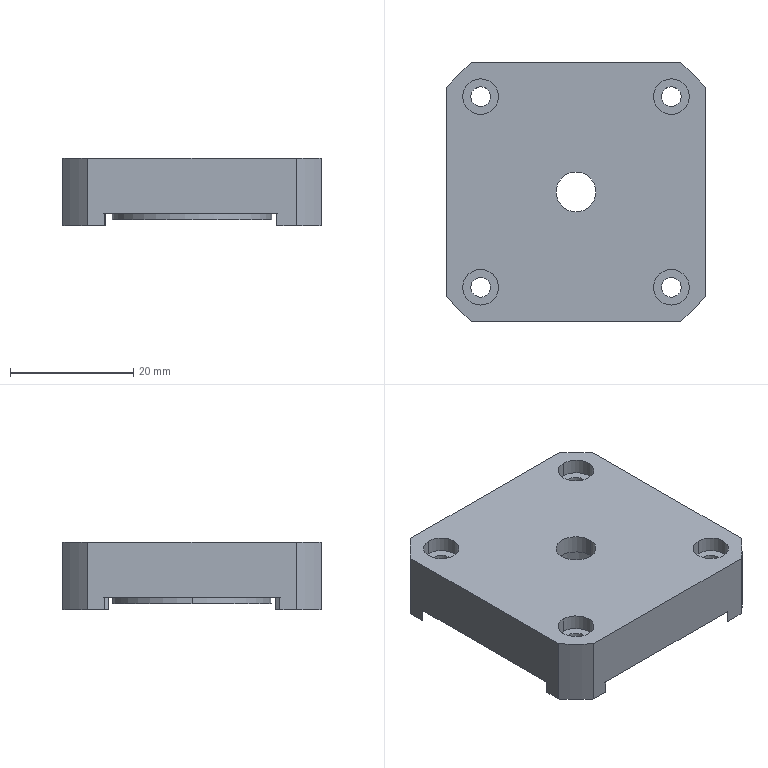Part | SolidWorks | features BaseBody 1 | 1 solid | 74 faces | box 42 x 42 x 11 mm | volume 9125 mm3 | cylinder 40 | plane 34 | commonest cylinder face diameters 3.2 x8 5.8 x8 7 x6 50.4 x4 54 x4 6.5 x2